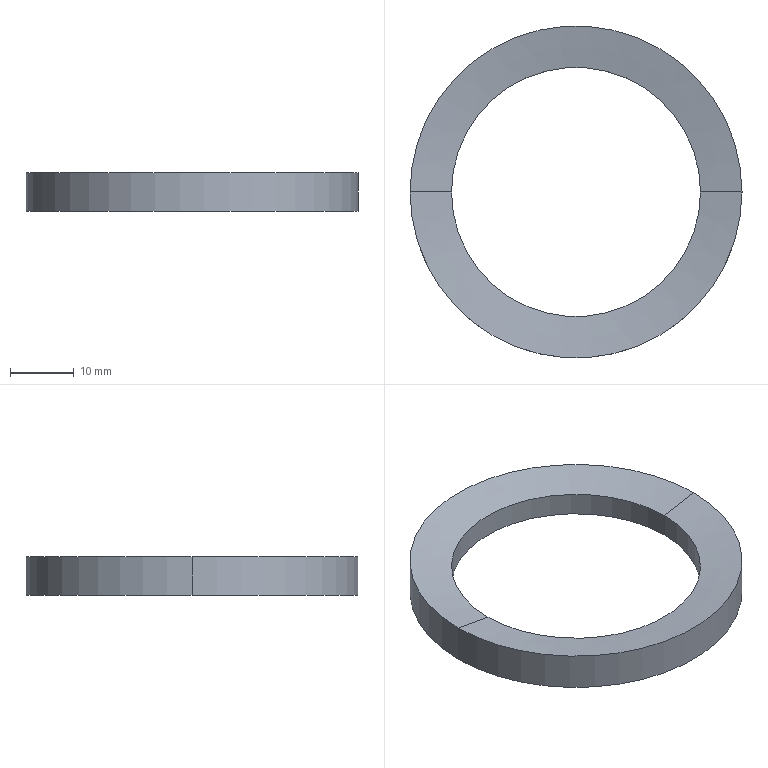Part | SolidWorks | features Extrusion 1, ICE 1, MirrorPattern 1 | 1 solid | 8 faces | box 52 x 52 x 6 mm | volume 4561 mm3 | cone 4 | cylinder 4 | commonest cylinder face diameters 39 x2 52 x2
STEP:
#1=CARTESIAN_POINT('',(-19.5,0.,-1.854));
#2=VERTEX_POINT('',#1);
#3=CARTESIAN_POINT('',(19.5,0.,-1.854));
#4=VERTEX_POINT('',#3);
#5=CARTESIAN_POINT('',(0.,0.,-1.854));
#6=DIRECTION('',(0.,0.,-1.));
#7=DIRECTION('',(-1.,0.,0.));
#8=AXIS2_PLACEMENT_3D('',#5,#6,#7);
#9=CIRCLE('',#8,19.5);
#10=EDGE_CURVE('',#2,#4,#9,.T.);
#11=ORIENTED_EDGE('',*,*,#10,.F.);
#12=CARTESIAN_POINT('',(-26.,0.,-3.));
#13=VERTEX_POINT('',#12);
#14=CARTESIAN_POINT('',(-26.,0.,-3.));
#15=DIRECTION('',(-0.9848,0.,-0.1736));
#16=VECTOR('',#15,1000.);
#17=LINE('',#14,#16);
#18=EDGE_CURVE('',#2,#13,#17,.T.);
#19=ORIENTED_EDGE('',*,*,#18,.T.);
#20=CARTESIAN_POINT('',(26.,0.,-3.));
#21=VERTEX_POINT('',#20);
#22=CARTESIAN_POINT('',(0.,0.,-3.));
#23=DIRECTION('',(0.,0.,1.));
#24=DIRECTION('',(1.,0.,0.));
#25=AXIS2_PLACEMENT_3D('',#22,#23,#24);
#26=CIRCLE('',#25,26.);
#27=EDGE_CURVE('',#21,#13,#26,.T.);
#28=ORIENTED_EDGE('',*,*,#27,.F.);
#29=CARTESIAN_POINT('',(26.,0.,-3.));
#30=DIRECTION('',(0.9848,0.,-0.1736));
#31=VECTOR('',#30,1000.);
#32=LINE('',#29,#31);
#33=EDGE_CURVE('',#4,#21,#32,.T.);
#34=ORIENTED_EDGE('',*,*,#33,.F.);
#35=EDGE_LOOP('',(#11,#19,#28,#34));
#36=FACE_OUTER_BOUND('',#35,.T.);
#37=CARTESIAN_POINT('',(0.,0.,-3.));
#38=DIRECTION('',(0.,0.,-1.));
#39=DIRECTION('',(1.,0.,0.));
#40=AXIS2_PLACEMENT_3D('',#37,#38,#39);
#41=CONICAL_SURFACE('',#40,26.,1.396);
#42=ADVANCED_FACE('',(#36),#41,.F.);
#43=CARTESIAN_POINT('',(19.5,0.,1.854));
#44=VERTEX_POINT('',#43);
#45=CARTESIAN_POINT('',(-19.5,0.,1.854));
#46=VERTEX_POINT('',#45);
#47=CARTESIAN_POINT('',(0.,0.,1.854));
#48=DIRECTION('',(0.,0.,-1.));
#49=DIRECTION('',(1.,0.,0.));
#50=AXIS2_PLACEMENT_3D('',#47,#48,#49);
#51=CIRCLE('',#50,19.5);
#52=EDGE_CURVE('',#44,#46,#51,.T.);
#53=ORIENTED_EDGE('',*,*,#52,.T.);
#54=CARTESIAN_POINT('',(-26.,0.,3.));
#55=VERTEX_POINT('',#54);
#56=CARTESIAN_POINT('',(-26.,0.,3.));
#57=DIRECTION('',(-0.9848,0.,0.1736));
#58=VECTOR('',#57,1000.);
#59=LINE('',#56,#58);
#60=EDGE_CURVE('',#46,#55,#59,.T.);
#61=ORIENTED_EDGE('',*,*,#60,.T.);
#62=CARTESIAN_POINT('',(26.,0.,3.));
#63=VERTEX_POINT('',#62);
#64=CARTESIAN_POINT('',(0.,0.,3.));
#65=DIRECTION('',(0.,0.,1.));
#66=DIRECTION('',(1.,0.,0.));
#67=AXIS2_PLACEMENT_3D('',#64,#65,#66);
#68=CIRCLE('',#67,26.);
#69=EDGE_CURVE('',#55,#63,#68,.T.);
#70=ORIENTED_EDGE('',*,*,#69,.T.);
#71=CARTESIAN_POINT('',(26.,0.,3.));
#72=DIRECTION('',(0.9848,0.,0.1736));
#73=VECTOR('',#72,1000.);
#74=LINE('',#71,#73);
#75=EDGE_CURVE('',#44,#63,#74,.T.);
#76=ORIENTED_EDGE('',*,*,#75,.F.);
#77=EDGE_LOOP('',(#53,#61,#70,#76));
#78=FACE_OUTER_BOUND('',#77,.T.);
#79=CARTESIAN_POINT('',(0.,0.,3.));
#80=DIRECTION('',(0.,0.,1.));
#81=DIRECTION('',(1.,0.,0.));
#82=AXIS2_PLACEMENT_3D('',#79,#80,#81);
#83=CONICAL_SURFACE('',#82,26.,1.396);
#84=ADVANCED_FACE('',(#78),#83,.F.);
#85=CARTESIAN_POINT('',(0.,0.,3.));
#86=DIRECTION('',(0.,0.,1.));
#87=DIRECTION('',(1.,0.,0.));
#88=AXIS2_PLACEMENT_3D('',#85,#86,#87);
#89=CIRCLE('',#88,26.);
#90=EDGE_CURVE('',#63,#55,#89,.T.);
#91=ORIENTED_EDGE('',*,*,#90,.F.);
#92=CARTESIAN_POINT('',(26.,0.,3.));
#93=DIRECTION('',(0.,0.,-1.));
#94=VECTOR('',#93,1000.);
#95=LINE('',#92,#94);
#96=EDGE_CURVE('',#63,#21,#95,.T.);
#97=ORIENTED_EDGE('',*,*,#96,.T.);
#98=ORIENTED_EDGE('',*,*,#27,.T.);
#99=CARTESIAN_POINT('',(-26.,0.,3.));
#100=DIRECTION('',(0.,0.,-1.));
#101=VECTOR('',#100,1000.);
#102=LINE('',#99,#101);
#103=EDGE_CURVE('',#55,#13,#102,.T.);
#104=ORIENTED_EDGE('',*,*,#103,.F.);
#105=EDGE_LOOP('',(#91,#97,#98,#104));
#106=FACE_OUTER_BOUND('',#105,.T.);
#107=CARTESIAN_POINT('',(0.,0.,3.));
#108=DIRECTION('',(0.,0.,-1.));
#109=DIRECTION('',(-1.,0.,0.));
#110=AXIS2_PLACEMENT_3D('',#107,#108,#109);
#111=CYLINDRICAL_SURFACE('',#110,26.);
#112=ADVANCED_FACE('',(#106),#111,.T.);
#113=ORIENTED_EDGE('',*,*,#52,.F.);
#114=CARTESIAN_POINT('',(19.5,0.,3.));
#115=DIRECTION('',(0.,0.,-1.));
#116=VECTOR('',#115,1000.);
#117=LINE('',#114,#116);
#118=EDGE_CURVE('',#44,#4,#117,.T.);
#119=ORIENTED_EDGE('',*,*,#118,.T.);
#120=CARTESIAN_POINT('',(0.,0.,-1.854));
#121=DIRECTION('',(0.,0.,-1.));
#122=DIRECTION('',(-1.,0.,0.));
#123=AXIS2_PLACEMENT_3D('',#120,#121,#122);
#124=CIRCLE('',#123,19.5);
#125=EDGE_CURVE('',#4,#2,#124,.T.);
#126=ORIENTED_EDGE('',*,*,#125,.T.);
#127=CARTESIAN_POINT('',(-19.5,0.,3.));
#128=DIRECTION('',(0.,0.,-1.));
#129=VECTOR('',#128,1000.);
#130=LINE('',#127,#129);
#131=EDGE_CURVE('',#46,#2,#130,.T.);
#132=ORIENTED_EDGE('',*,*,#131,.F.);
#133=EDGE_LOOP('',(#113,#119,#126,#132));
#134=FACE_OUTER_BOUND('',#133,.T.);
#135=CARTESIAN_POINT('',(0.,0.,3.));
#136=DIRECTION('',(0.,0.,-1.));
#137=DIRECTION('',(-1.,0.,0.));
#138=AXIS2_PLACEMENT_3D('',#135,#136,#137);
#139=CYLINDRICAL_SURFACE('',#138,19.5);
#140=ADVANCED_FACE('',(#134),#139,.F.);
#141=ORIENTED_EDGE('',*,*,#118,.F.);
#142=CARTESIAN_POINT('',(0.,0.,1.854));
#143=DIRECTION('',(0.,0.,-1.));
#144=DIRECTION('',(1.,0.,0.));
#145=AXIS2_PLACEMENT_3D('',#142,#143,#144);
#146=CIRCLE('',#145,19.5);
#147=EDGE_CURVE('',#46,#44,#146,.T.);
#148=ORIENTED_EDGE('',*,*,#147,.F.);
#149=ORIENTED_EDGE('',*,*,#131,.T.);
#150=ORIENTED_EDGE('',*,*,#10,.T.);
#151=EDGE_LOOP('',(#141,#148,#149,#150));
#152=FACE_OUTER_BOUND('',#151,.T.);
#153=CARTESIAN_POINT('',(0.,0.,3.));
#154=DIRECTION('',(0.,0.,-1.));
#155=DIRECTION('',(-1.,0.,0.));
#156=AXIS2_PLACEMENT_3D('',#153,#154,#155);
#157=CYLINDRICAL_SURFACE('',#156,19.5);
#158=ADVANCED_FACE('',(#152),#157,.F.);
#159=ORIENTED_EDGE('',*,*,#96,.F.);
#160=ORIENTED_EDGE('',*,*,#69,.F.);
#161=ORIENTED_EDGE('',*,*,#103,.T.);
#162=CARTESIAN_POINT('',(0.,0.,-3.));
#163=DIRECTION('',(0.,0.,1.));
#164=DIRECTION('',(1.,0.,0.));
#165=AXIS2_PLACEMENT_3D('',#162,#163,#164);
#166=CIRCLE('',#165,26.);
#167=EDGE_CURVE('',#13,#21,#166,.T.);
#168=ORIENTED_EDGE('',*,*,#167,.T.);
#169=EDGE_LOOP('',(#159,#160,#161,#168));
#170=FACE_OUTER_BOUND('',#169,.T.);
#171=CARTESIAN_POINT('',(0.,0.,3.));
#172=DIRECTION('',(0.,0.,-1.));
#173=DIRECTION('',(-1.,0.,0.));
#174=AXIS2_PLACEMENT_3D('',#171,#172,#173);
#175=CYLINDRICAL_SURFACE('',#174,26.);
#176=ADVANCED_FACE('',(#170),#175,.T.);
#177=ORIENTED_EDGE('',*,*,#60,.F.);
#178=ORIENTED_EDGE('',*,*,#147,.T.);
#179=ORIENTED_EDGE('',*,*,#75,.T.);
#180=ORIENTED_EDGE('',*,*,#90,.T.);
#181=EDGE_LOOP('',(#177,#178,#179,#180));
#182=FACE_OUTER_BOUND('',#181,.T.);
#183=CARTESIAN_POINT('',(0.,0.,3.));
#184=DIRECTION('',(0.,0.,1.));
#185=DIRECTION('',(1.,0.,0.));
#186=AXIS2_PLACEMENT_3D('',#183,#184,#185);
#187=CONICAL_SURFACE('',#186,26.,1.396);
#188=ADVANCED_FACE('',(#182),#187,.F.);
#189=ORIENTED_EDGE('',*,*,#18,.F.);
#190=ORIENTED_EDGE('',*,*,#125,.F.);
#191=ORIENTED_EDGE('',*,*,#33,.T.);
#192=ORIENTED_EDGE('',*,*,#167,.F.);
#193=EDGE_LOOP('',(#189,#190,#191,#192));
#194=FACE_OUTER_BOUND('',#193,.T.);
#195=CARTESIAN_POINT('',(0.,0.,-3.));
#196=DIRECTION('',(0.,0.,-1.));
#197=DIRECTION('',(1.,0.,0.));
#198=AXIS2_PLACEMENT_3D('',#195,#196,#197);
#199=CONICAL_SURFACE('',#198,26.,1.396);
#200=ADVANCED_FACE('',(#194),#199,.F.);
#201=CLOSED_SHELL('',(#42,#84,#112,#140,#158,#176,#188,#200));
#202=MANIFOLD_SOLID_BREP('',#201);
#203=CARTESIAN_POINT('',(0.,0.,0.));
#204=DIRECTION('',(0.,0.,1.));
#205=DIRECTION('',(1.,0.,0.));
#206=AXIS2_PLACEMENT_3D('',#203,#204,#205);
#207=(LENGTH_UNIT()NAMED_UNIT(*)SI_UNIT(.MILLI.,.METRE.));
#208=UNCERTAINTY_MEASURE_WITH_UNIT(LENGTH_MEASURE(0.00001),#207,'','');
#209=(NAMED_UNIT(*)PLANE_ANGLE_UNIT()SI_UNIT($,.RADIAN.));
#210=(NAMED_UNIT(*)SI_UNIT($,.STERADIAN.)SOLID_ANGLE_UNIT());
#211=(GEOMETRIC_REPRESENTATION_CONTEXT(3)GLOBAL_UNCERTAINTY_ASSIGNED_CONTEXT((#208))GLOBAL_UNIT_ASSIGNED_CONTEXT((#207,#209,#210))REPRESENTATION_CONTEXT('',''));
#212=ADVANCED_BREP_SHAPE_REPRESENTATION('',(#202,#206),#211);